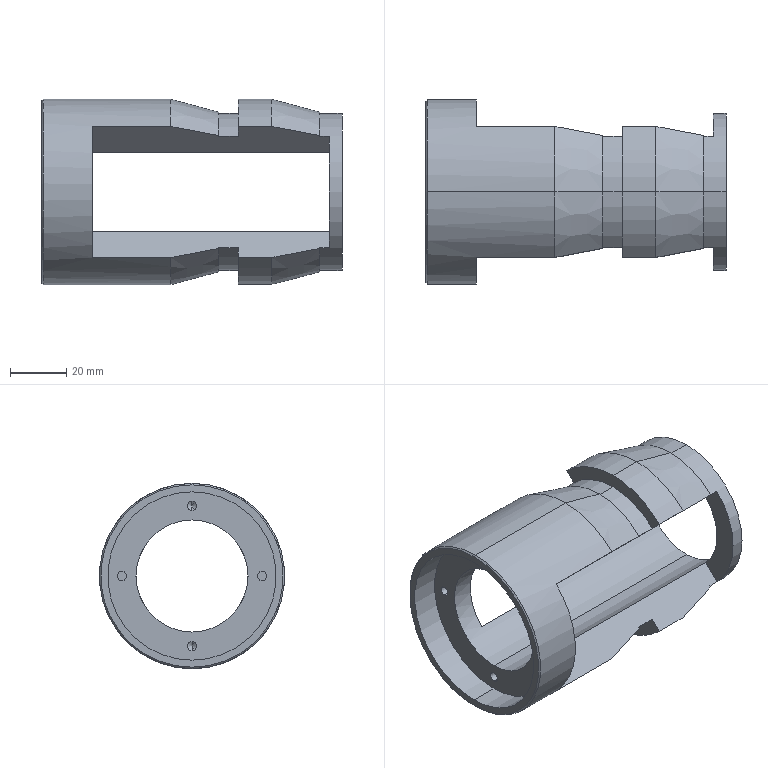Part | SolidWorks | features Chamfer 1, HoleWzd 1, MirrorPattern 1, RefAxis 1, RevCut 1, Revolution 1 | 1 solid | 51 faces | box 107 x 66 x 66 mm | volume 107081 mm3 | cylinder 22 | plane 17 | cone 12 | commonest cylinder face diameters 3.3 x8 56 x5 66 x5 40 x2 60 x2